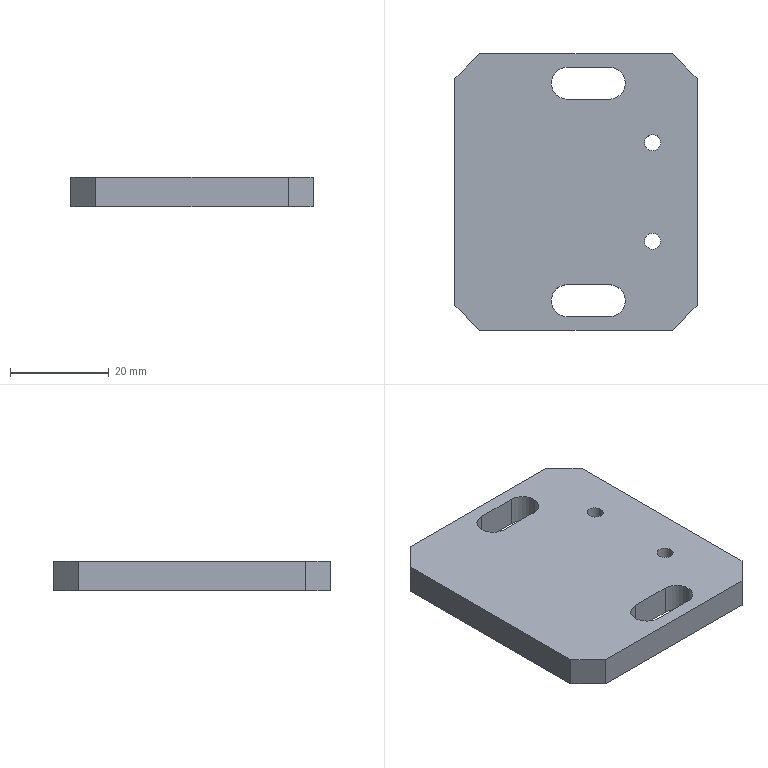Part | STEP file | solid 60 | 1 solid | 20 faces | box 49 x 56 x 6 mm | volume 15004 mm3 | plane 14 | cylinder 6 | commonest cylinder face diameters 6.5 x4 3.242 x2